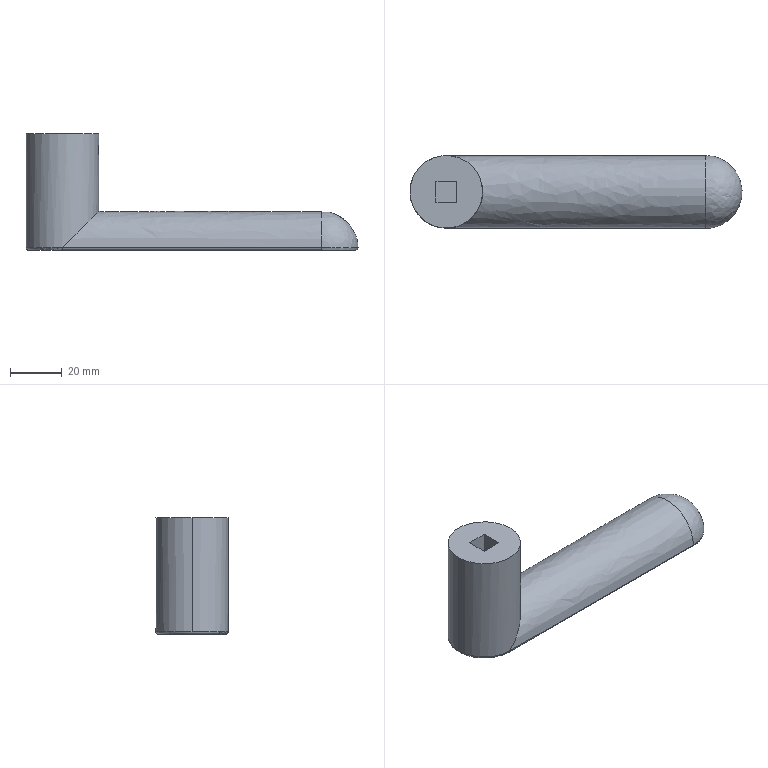Part | SolidWorks | features ICE 5, Cut 2, Blend 1, Extrusion 1, Fillet 1, HoleWzd 1, NetBlend 1 | 1 solid | 17 faces | box 128.025 x 28 x 45 mm | volume 59416 mm3 | plane 7 | cylinder 6 | spline 3 | torus 1 | commonest cylinder face diameters 2 x2 4.2 x2 28 x2
STEP:
#1=CARTESIAN_POINT('',(14.,0.,36.4));
#2=VERTEX_POINT('',#1);
#3=CARTESIAN_POINT('',(14.,0.,40.6));
#4=VERTEX_POINT('',#3);
#5=CARTESIAN_POINT('',(14.,0.,36.4));
#6=CARTESIAN_POINT('',(14.,-0.2742,36.4));
#7=CARTESIAN_POINT('',(13.991,-0.5509,36.455));
#8=CARTESIAN_POINT('',(13.97,-0.93,36.612));
#9=CARTESIAN_POINT('',(13.961,-1.052,36.677));
#10=CARTESIAN_POINT('',(13.942,-1.282,36.831));
#11=CARTESIAN_POINT('',(13.931,-1.387,36.917));
#12=CARTESIAN_POINT('',(13.911,-1.581,37.111));
#13=CARTESIAN_POINT('',(13.9,-1.669,37.219));
#14=CARTESIAN_POINT('',(13.881,-1.822,37.446));
#15=CARTESIAN_POINT('',(13.872,-1.886,37.567));
#16=CARTESIAN_POINT('',(13.858,-1.992,37.821));
#17=CARTESIAN_POINT('',(13.852,-2.033,37.954));
#18=CARTESIAN_POINT('',(13.844,-2.086,38.223));
#19=CARTESIAN_POINT('',(13.842,-2.1,38.36));
#20=CARTESIAN_POINT('',(13.842,-2.1,38.637));
#21=CARTESIAN_POINT('',(13.844,-2.087,38.774));
#22=CARTESIAN_POINT('',(13.852,-2.033,39.043));
#23=CARTESIAN_POINT('',(13.858,-1.993,39.176));
#24=CARTESIAN_POINT('',(13.872,-1.888,39.43));
#25=CARTESIAN_POINT('',(13.881,-1.823,39.551));
#26=CARTESIAN_POINT('',(13.9,-1.671,39.779));
#27=CARTESIAN_POINT('',(13.911,-1.583,39.887));
#28=CARTESIAN_POINT('',(13.942,-1.293,40.177));
#29=CARTESIAN_POINT('',(13.962,-1.059,40.334));
#30=CARTESIAN_POINT('',(13.991,-0.5539,40.544));
#31=CARTESIAN_POINT('',(14.,-0.2779,40.6));
#32=CARTESIAN_POINT('',(14.,0.,40.6));
#33=B_SPLINE_CURVE_WITH_KNOTS('',3,(#5,#6,#7,#8,#9,#10,#11,#12,#13,#14,#15,#16,#17,#18,#19,#20,#21,#22,#23,#24,#25,#26,#27,#28,#29,#30,#31,#32),.UNSPECIFIED.,.F.,.F.,(4,2,2,2,2,2,2,2,2,2,2,2,2,4),(0.006575,0.007396,0.007807,0.008218,0.008629,0.00904,0.009451,0.009861,0.01027,0.01068,0.01109,0.0115,0.01233,0.01315),.UNSPECIFIED.);
#34=EDGE_CURVE('',#2,#4,#33,.T.);
#35=ORIENTED_EDGE('',*,*,#34,.F.);
#36=CARTESIAN_POINT('',(4.,0.,36.4));
#37=VERTEX_POINT('',#36);
#38=CARTESIAN_POINT('',(4.,0.,36.4));
#39=DIRECTION('',(-1.,0.,0.));
#40=VECTOR('',#39,1000.);
#41=LINE('',#38,#40);
#42=EDGE_CURVE('',#2,#37,#41,.T.);
#43=ORIENTED_EDGE('',*,*,#42,.T.);
#44=CARTESIAN_POINT('',(4.,0.,40.6));
#45=VERTEX_POINT('',#44);
#46=CARTESIAN_POINT('',(4.,0.,38.5));
#47=DIRECTION('',(-1.,0.,0.));
#48=DIRECTION('',(0.,0.,1.));
#49=AXIS2_PLACEMENT_3D('',#46,#47,#48);
#50=CIRCLE('',#49,2.1);
#51=EDGE_CURVE('',#37,#45,#50,.T.);
#52=ORIENTED_EDGE('',*,*,#51,.T.);
#53=CARTESIAN_POINT('',(4.,0.,40.6));
#54=DIRECTION('',(-1.,0.,0.));
#55=VECTOR('',#54,1000.);
#56=LINE('',#53,#55);
#57=EDGE_CURVE('',#4,#45,#56,.T.);
#58=ORIENTED_EDGE('',*,*,#57,.F.);
#59=EDGE_LOOP('',(#35,#43,#52,#58));
#60=FACE_OUTER_BOUND('',#59,.T.);
#61=CARTESIAN_POINT('',(4.,0.,38.5));
#62=DIRECTION('',(-1.,0.,0.));
#63=DIRECTION('',(0.,0.,1.));
#64=AXIS2_PLACEMENT_3D('',#61,#62,#63);
#65=CYLINDRICAL_SURFACE('',#64,2.1);
#66=ADVANCED_FACE('',(#60),#65,.F.);
#67=CARTESIAN_POINT('',(14.,0.,45.));
#68=VERTEX_POINT('',#67);
#69=CARTESIAN_POINT('',(-14.,0.,45.));
#70=VERTEX_POINT('',#69);
#71=CARTESIAN_POINT('',(0.,0.,45.));
#72=DIRECTION('',(0.,0.,1.));
#73=DIRECTION('',(1.,0.,0.));
#74=AXIS2_PLACEMENT_3D('',#71,#72,#73);
#75=CIRCLE('',#74,14.);
#76=EDGE_CURVE('',#68,#70,#75,.T.);
#77=ORIENTED_EDGE('',*,*,#76,.F.);
#78=CARTESIAN_POINT('',(14.,0.,45.));
#79=DIRECTION('',(0.,0.,-1.));
#80=VECTOR('',#79,1000.);
#81=LINE('',#78,#80);
#82=EDGE_CURVE('',#68,#4,#81,.T.);
#83=ORIENTED_EDGE('',*,*,#82,.T.);
#84=CARTESIAN_POINT('',(14.,0.,40.6));
#85=CARTESIAN_POINT('',(14.,0.139,40.6));
#86=CARTESIAN_POINT('',(13.998,0.2756,40.586));
#87=CARTESIAN_POINT('',(13.99,0.5443,40.533));
#88=CARTESIAN_POINT('',(13.984,0.6777,40.492));
#89=CARTESIAN_POINT('',(13.97,0.932,40.387));
#90=CARTESIAN_POINT('',(13.961,1.053,40.322));
#91=CARTESIAN_POINT('',(13.942,1.281,40.17));
#92=CARTESIAN_POINT('',(13.931,1.389,40.081));
#93=CARTESIAN_POINT('',(13.9,1.679,39.791));
#94=CARTESIAN_POINT('',(13.88,1.835,39.557));
#95=CARTESIAN_POINT('',(13.85,2.045,39.052));
#96=CARTESIAN_POINT('',(13.842,2.1,38.775));
#97=CARTESIAN_POINT('',(13.842,2.1,38.364));
#98=CARTESIAN_POINT('',(13.844,2.086,38.224));
#99=CARTESIAN_POINT('',(13.852,2.033,37.955));
#100=CARTESIAN_POINT('',(13.858,1.993,37.824));
#101=CARTESIAN_POINT('',(13.872,1.887,37.569));
#102=CARTESIAN_POINT('',(13.881,1.822,37.447));
#103=CARTESIAN_POINT('',(13.9,1.67,37.219));
#104=CARTESIAN_POINT('',(13.911,1.583,37.113));
#105=CARTESIAN_POINT('',(13.931,1.387,36.917));
#106=CARTESIAN_POINT('',(13.942,1.281,36.831));
#107=CARTESIAN_POINT('',(13.961,1.054,36.679));
#108=CARTESIAN_POINT('',(13.97,0.9311,36.613));
#109=CARTESIAN_POINT('',(13.984,0.6769,36.507));
#110=CARTESIAN_POINT('',(13.99,0.546,36.468));
#111=CARTESIAN_POINT('',(13.998,0.2765,36.414));
#112=CARTESIAN_POINT('',(14.,0.1372,36.4));
#113=CARTESIAN_POINT('',(14.,0.,36.4));
#114=B_SPLINE_CURVE_WITH_KNOTS('',3,(#84,#85,#86,#87,#88,#89,#90,#91,#92,#93,#94,#95,#96,#97,#98,#99,#100,#101,#102,#103,#104,#105,#106,#107,#108,#109,#110,#111,#112,#113),.UNSPECIFIED.,.F.,.F.,(4,2,2,2,2,2,2,2,2,2,2,2,2,2,4),(0.,0.0004109,0.0008219,0.001233,0.001644,0.002466,0.003287,0.003698,0.004109,0.00452,0.004931,0.005342,0.005753,0.006164,0.006575),.UNSPECIFIED.);
#115=EDGE_CURVE('',#4,#2,#114,.T.);
#116=ORIENTED_EDGE('',*,*,#115,.T.);
#117=CARTESIAN_POINT('',(14.,0.,15.));
#118=VERTEX_POINT('',#117);
#119=CARTESIAN_POINT('',(14.,0.,45.));
#120=DIRECTION('',(0.,0.,-1.));
#121=VECTOR('',#120,1000.);
#122=LINE('',#119,#121);
#123=EDGE_CURVE('',#2,#118,#122,.T.);
#124=ORIENTED_EDGE('',*,*,#123,.T.);
#125=CARTESIAN_POINT('',(0.,14.,1.));
#126=VERTEX_POINT('',#125);
#127=CARTESIAN_POINT('',(14.,0.,15.));
#128=CARTESIAN_POINT('',(14.,0.5649,15.));
#129=CARTESIAN_POINT('',(13.966,1.123,14.966));
#130=CARTESIAN_POINT('',(13.833,2.228,14.832));
#131=CARTESIAN_POINT('',(13.733,2.777,14.732));
#132=CARTESIAN_POINT('',(13.475,3.836,14.475));
#133=CARTESIAN_POINT('',(13.318,4.347,14.319));
#134=CARTESIAN_POINT('',(13.045,5.088,14.046));
#135=CARTESIAN_POINT('',(12.948,5.331,13.949));
#136=CARTESIAN_POINT('',(12.741,5.808,13.741));
#137=CARTESIAN_POINT('',(12.631,6.044,13.631));
#138=CARTESIAN_POINT('',(12.057,7.189,13.056));
#139=CARTESIAN_POINT('',(11.524,8.007,12.523));
#140=CARTESIAN_POINT('',(10.637,9.115,11.637));
#141=CARTESIAN_POINT('',(10.325,9.466,11.325));
#142=CARTESIAN_POINT('',(9.683,10.122,10.684));
#143=CARTESIAN_POINT('',(9.354,10.426,10.354));
#144=CARTESIAN_POINT('',(8.342,11.278,9.341));
#145=CARTESIAN_POINT('',(7.636,11.764,8.635));
#146=CARTESIAN_POINT('',(6.537,12.387,7.537));
#147=CARTESIAN_POINT('',(6.162,12.578,7.163));
#148=CARTESIAN_POINT('',(5.411,12.918,6.413));
#149=CARTESIAN_POINT('',(5.034,13.07,6.035));
#150=CARTESIAN_POINT('',(3.895,13.471,4.895));
#151=CARTESIAN_POINT('',(3.129,13.669,4.126));
#152=CARTESIAN_POINT('',(1.578,13.933,2.573));
#153=CARTESIAN_POINT('',(0.7944,14.,1.79));
#154=CARTESIAN_POINT('',(0.,14.,1.));
#155=B_SPLINE_CURVE_WITH_KNOTS('',3,(#127,#128,#129,#130,#131,#132,#133,#134,#135,#136,#137,#138,#139,#140,#141,#142,#143,#144,#145,#146,#147,#148,#149,#150,#151,#152,#153,#154),.UNSPECIFIED.,.F.,.F.,(4,2,2,2,2,2,2,2,2,2,2,2,2,4),(0.02682,0.0285,0.03018,0.03186,0.0327,0.03354,0.0369,0.03858,0.04026,0.04362,0.0453,0.04698,0.05034,0.0537),.UNSPECIFIED.);
#156=EDGE_CURVE('',#118,#126,#155,.T.);
#157=ORIENTED_EDGE('',*,*,#156,.T.);
#158=CARTESIAN_POINT('',(-14.,0.,1.));
#159=VERTEX_POINT('',#158);
#160=CARTESIAN_POINT('',(0.,0.,1.));
#161=DIRECTION('',(0.,0.,1.));
#162=DIRECTION('',(1.,0.,0.));
#163=AXIS2_PLACEMENT_3D('',#160,#161,#162);
#164=CIRCLE('',#163,14.);
#165=EDGE_CURVE('',#126,#159,#164,.T.);
#166=ORIENTED_EDGE('',*,*,#165,.T.);
#167=CARTESIAN_POINT('',(-14.,0.,45.));
#168=DIRECTION('',(0.,0.,-1.));
#169=VECTOR('',#168,1000.);
#170=LINE('',#167,#169);
#171=EDGE_CURVE('',#70,#159,#170,.T.);
#172=ORIENTED_EDGE('',*,*,#171,.F.);
#173=EDGE_LOOP('',(#77,#83,#116,#124,#157,#166,#172));
#174=FACE_OUTER_BOUND('',#173,.T.);
#175=CARTESIAN_POINT('',(0.,0.,45.));
#176=DIRECTION('',(0.,0.,-1.));
#177=DIRECTION('',(-1.,0.,0.));
#178=AXIS2_PLACEMENT_3D('',#175,#176,#177);
#179=CYLINDRICAL_SURFACE('',#178,14.);
#180=ADVANCED_FACE('',(#174),#179,.T.);
#181=ORIENTED_EDGE('',*,*,#82,.F.);
#182=CARTESIAN_POINT('',(0.,0.,45.));
#183=DIRECTION('',(0.,0.,1.));
#184=DIRECTION('',(1.,0.,0.));
#185=AXIS2_PLACEMENT_3D('',#182,#183,#184);
#186=CIRCLE('',#185,14.);
#187=EDGE_CURVE('',#70,#68,#186,.T.);
#188=ORIENTED_EDGE('',*,*,#187,.F.);
#189=ORIENTED_EDGE('',*,*,#171,.T.);
#190=CARTESIAN_POINT('',(0.,-14.,1.));
#191=VERTEX_POINT('',#190);
#192=CARTESIAN_POINT('',(0.,0.,1.));
#193=DIRECTION('',(0.,0.,1.));
#194=DIRECTION('',(1.,0.,0.));
#195=AXIS2_PLACEMENT_3D('',#192,#193,#194);
#196=CIRCLE('',#195,14.);
#197=EDGE_CURVE('',#159,#191,#196,.T.);
#198=ORIENTED_EDGE('',*,*,#197,.T.);
#199=CARTESIAN_POINT('',(0.,-14.,1.));
#200=CARTESIAN_POINT('',(0.7932,-14.,1.789));
#201=CARTESIAN_POINT('',(1.584,-13.933,2.578));
#202=CARTESIAN_POINT('',(3.152,-13.664,4.149));
#203=CARTESIAN_POINT('',(3.929,-13.462,4.928));
#204=CARTESIAN_POINT('',(5.462,-12.916,6.464));
#205=CARTESIAN_POINT('',(6.209,-12.575,7.21));
#206=CARTESIAN_POINT('',(7.66,-11.748,8.659));
#207=CARTESIAN_POINT('',(8.363,-11.263,9.362));
#208=CARTESIAN_POINT('',(9.378,-10.404,10.378));
#209=CARTESIAN_POINT('',(9.71,-10.096,10.711));
#210=CARTESIAN_POINT('',(10.348,-9.441,11.348));
#211=CARTESIAN_POINT('',(10.654,-9.095,11.654));
#212=CARTESIAN_POINT('',(11.241,-8.359,12.24));
#213=CARTESIAN_POINT('',(11.52,-7.97,12.52));
#214=CARTESIAN_POINT('',(12.05,-7.144,13.049));
#215=CARTESIAN_POINT('',(12.301,-6.705,13.3));
#216=CARTESIAN_POINT('',(12.756,-5.792,13.756));
#217=CARTESIAN_POINT('',(12.961,-5.318,13.962));
#218=CARTESIAN_POINT('',(13.234,-4.576,14.234));
#219=CARTESIAN_POINT('',(13.318,-4.324,14.318));
#220=CARTESIAN_POINT('',(13.474,-3.809,14.474));
#221=CARTESIAN_POINT('',(13.546,-3.546,14.546));
#222=CARTESIAN_POINT('',(13.866,-2.22,14.865));
#223=CARTESIAN_POINT('',(14.,-1.128,15.));
#224=CARTESIAN_POINT('',(14.,0.,15.));
#225=B_SPLINE_CURVE_WITH_KNOTS('',3,(#199,#200,#201,#202,#203,#204,#205,#206,#207,#208,#209,#210,#211,#212,#213,#214,#215,#216,#217,#218,#219,#220,#221,#222,#223,#224),.UNSPECIFIED.,.F.,.F.,(4,2,2,2,2,2,2,2,2,2,2,2,4),(-0.00002366,0.003332,0.006687,0.01004,0.0134,0.01508,0.01675,0.01843,0.02011,0.02179,0.02263,0.02346,0.02682),.UNSPECIFIED.);
#226=EDGE_CURVE('',#191,#118,#225,.T.);
#227=ORIENTED_EDGE('',*,*,#226,.T.);
#228=ORIENTED_EDGE('',*,*,#123,.F.);
#229=ORIENTED_EDGE('',*,*,#34,.T.);
#230=EDGE_LOOP('',(#181,#188,#189,#198,#227,#228,#229));
#231=FACE_OUTER_BOUND('',#230,.T.);
#232=CARTESIAN_POINT('',(0.,0.,45.));
#233=DIRECTION('',(0.,0.,-1.));
#234=DIRECTION('',(-1.,0.,0.));
#235=AXIS2_PLACEMENT_3D('',#232,#233,#234);
#236=CYLINDRICAL_SURFACE('',#235,14.);
#237=ADVANCED_FACE('',(#231),#236,.T.);
#238=ORIENTED_EDGE('',*,*,#187,.T.);
#239=ORIENTED_EDGE('',*,*,#76,.T.);
#240=EDGE_LOOP('',(#238,#239));
#241=FACE_OUTER_BOUND('',#240,.T.);
#242=CARTESIAN_POINT('',(4.,-4.,45.));
#243=VERTEX_POINT('',#242);
#244=CARTESIAN_POINT('',(-4.,-4.,45.));
#245=VERTEX_POINT('',#244);
#246=CARTESIAN_POINT('',(-4.,-4.,45.));
#247=DIRECTION('',(-1.,0.,0.));
#248=VECTOR('',#247,1000.);
#249=LINE('',#246,#248);
#250=EDGE_CURVE('',#243,#245,#249,.T.);
#251=ORIENTED_EDGE('',*,*,#250,.T.);
#252=CARTESIAN_POINT('',(-4.,4.,45.));
#253=VERTEX_POINT('',#252);
#254=CARTESIAN_POINT('',(-4.,-4.,45.));
#255=DIRECTION('',(0.,1.,0.));
#256=VECTOR('',#255,1000.);
#257=LINE('',#254,#256);
#258=EDGE_CURVE('',#245,#253,#257,.T.);
#259=ORIENTED_EDGE('',*,*,#258,.T.);
#260=CARTESIAN_POINT('',(4.,4.,45.));
#261=VERTEX_POINT('',#260);
#262=CARTESIAN_POINT('',(-4.,4.,45.));
#263=DIRECTION('',(1.,0.,0.));
#264=VECTOR('',#263,1000.);
#265=LINE('',#262,#264);
#266=EDGE_CURVE('',#253,#261,#265,.T.);
#267=ORIENTED_EDGE('',*,*,#266,.T.);
#268=CARTESIAN_POINT('',(4.,-4.,45.));
#269=DIRECTION('',(0.,-1.,0.));
#270=VECTOR('',#269,1000.);
#271=LINE('',#268,#270);
#272=EDGE_CURVE('',#261,#243,#271,.T.);
#273=ORIENTED_EDGE('',*,*,#272,.T.);
#274=EDGE_LOOP('',(#251,#259,#267,#273));
#275=FACE_BOUND('',#274,.T.);
#276=CARTESIAN_POINT('',(0.,0.,45.));
#277=DIRECTION('',(0.,0.,1.));
#278=DIRECTION('',(1.,0.,0.));
#279=AXIS2_PLACEMENT_3D('',#276,#277,#278);
#280=PLANE('',#279);
#281=ADVANCED_FACE('',(#241,#275),#280,.T.);
#282=CARTESIAN_POINT('',(0.,13.,0.));
#283=VERTEX_POINT('',#282);
#284=CARTESIAN_POINT('',(99.976,13.,0.));
#285=VERTEX_POINT('',#284);
#286=CARTESIAN_POINT('',(100.,13.,0.));
#287=DIRECTION('',(1.,0.,0.));
#288=VECTOR('',#287,1000.);
#289=LINE('',#286,#288);
#290=EDGE_CURVE('',#283,#285,#289,.T.);
#291=ORIENTED_EDGE('',*,*,#290,.T.);
#292=CARTESIAN_POINT('',(99.977,-13.,0.));
#293=VERTEX_POINT('',#292);
#294=CARTESIAN_POINT('',(99.976,13.,0.));
#295=CARTESIAN_POINT('',(100.407,12.99,0.));
#296=CARTESIAN_POINT('',(100.838,12.982,0.));
#297=CARTESIAN_POINT('',(101.695,12.914,0.));
#298=CARTESIAN_POINT('',(102.123,12.858,0.));
#299=CARTESIAN_POINT('',(103.388,12.624,0.));
#300=CARTESIAN_POINT('',(104.203,12.383,0.));
#301=CARTESIAN_POINT('',(105.385,11.9,0.));
#302=CARTESIAN_POINT('',(105.773,11.718,0.));
#303=CARTESIAN_POINT('',(106.533,11.314,0.));
#304=CARTESIAN_POINT('',(106.9,11.094,0.));
#305=CARTESIAN_POINT('',(107.961,10.383,0.));
#306=CARTESIAN_POINT('',(108.618,9.843,0.));
#307=CARTESIAN_POINT('',(109.526,8.931,0.));
#308=CARTESIAN_POINT('',(109.815,8.61,0.));
#309=CARTESIAN_POINT('',(110.353,7.949,0.));
#310=CARTESIAN_POINT('',(110.605,7.606,0.));
#311=CARTESIAN_POINT('',(111.075,6.898,0.));
#312=CARTESIAN_POINT('',(111.293,6.533,0.));
#313=CARTESIAN_POINT('',(111.693,5.779,0.));
#314=CARTESIAN_POINT('',(111.877,5.388,0.));
#315=CARTESIAN_POINT('',(112.366,4.199,0.));
#316=CARTESIAN_POINT('',(112.609,3.386,0.));
#317=CARTESIAN_POINT('',(112.857,2.134,0.));
#318=CARTESIAN_POINT('',(112.92,1.711,0.));
#319=CARTESIAN_POINT('',(113.004,0.8554,0.));
#320=CARTESIAN_POINT('',(113.025,0.4269,0.));
#321=CARTESIAN_POINT('',(113.025,-0.8504,0.));
#322=CARTESIAN_POINT('',(112.94,-1.695,0.));
#323=CARTESIAN_POINT('',(112.691,-2.952,0.));
#324=CARTESIAN_POINT('',(112.587,-3.372,0.));
#325=CARTESIAN_POINT('',(112.34,-4.191,0.));
#326=CARTESIAN_POINT('',(112.198,-4.592,0.));
#327=CARTESIAN_POINT('',(111.714,-5.77,0.));
#328=CARTESIAN_POINT('',(111.316,-6.522,0.));
#329=CARTESIAN_POINT('',(110.365,-7.957,0.));
#330=CARTESIAN_POINT('',(109.827,-8.617,0.));
#331=CARTESIAN_POINT('',(108.93,-9.521,0.));
#332=CARTESIAN_POINT('',(108.616,-9.808,0.));
#333=CARTESIAN_POINT('',(107.957,-10.352,0.));
#334=CARTESIAN_POINT('',(107.61,-10.611,0.));
#335=CARTESIAN_POINT('',(106.546,-11.325,0.));
#336=CARTESIAN_POINT('',(105.798,-11.725,0.));
#337=CARTESIAN_POINT('',(104.223,-12.373,0.));
#338=CARTESIAN_POINT('',(103.392,-12.621,0.));
#339=CARTESIAN_POINT('',(102.125,-12.858,0.));
#340=CARTESIAN_POINT('',(101.697,-12.914,0.));
#341=CARTESIAN_POINT('',(100.839,-12.982,0.));
#342=CARTESIAN_POINT('',(100.408,-12.99,0.));
#343=CARTESIAN_POINT('',(99.977,-13.,0.));
#344=B_SPLINE_CURVE_WITH_KNOTS('',3,(#294,#295,#296,#297,#298,#299,#300,#301,#302,#303,#304,#305,#306,#307,#308,#309,#310,#311,#312,#313,#314,#315,#316,#317,#318,#319,#320,#321,#322,#323,#324,#325,#326,#327,#328,#329,#330,#331,#332,#333,#334,#335,#336,#337,#338,#339,#340,#341,#342,#343),.UNSPECIFIED.,.F.,.F.,(4,2,2,2,2,2,2,2,2,2,2,2,2,2,2,2,2,2,2,2,2,2,2,2,4),(0.,0.001292,0.002584,0.005168,0.00646,0.007752,0.01034,0.01163,0.01292,0.01421,0.0155,0.01809,0.01938,0.02067,0.02325,0.02455,0.02584,0.02842,0.03101,0.0323,0.03359,0.03617,0.03876,0.04005,0.04134),.UNSPECIFIED.);
#345=EDGE_CURVE('',#285,#293,#344,.T.);
#346=ORIENTED_EDGE('',*,*,#345,.T.);
#347=CARTESIAN_POINT('',(0.,-13.,0.));
#348=VERTEX_POINT('',#347);
#349=CARTESIAN_POINT('',(0.,-13.,0.));
#350=DIRECTION('',(-1.,0.,0.));
#351=VECTOR('',#350,1000.);
#352=LINE('',#349,#351);
#353=EDGE_CURVE('',#293,#348,#352,.T.);
#354=ORIENTED_EDGE('',*,*,#353,.T.);
#355=CARTESIAN_POINT('',(0.,0.,0.));
#356=DIRECTION('',(0.,0.,-1.));
#357=DIRECTION('',(1.,0.,0.));
#358=AXIS2_PLACEMENT_3D('',#355,#356,#357);
#359=CIRCLE('',#358,13.);
#360=EDGE_CURVE('',#348,#283,#359,.T.);
#361=ORIENTED_EDGE('',*,*,#360,.T.);
#362=EDGE_LOOP('',(#291,#346,#354,#361));
#363=FACE_OUTER_BOUND('',#362,.T.);
#364=CARTESIAN_POINT('',(0.,0.,0.));
#365=DIRECTION('',(0.,0.,1.));
#366=DIRECTION('',(1.,0.,0.));
#367=AXIS2_PLACEMENT_3D('',#364,#365,#366);
#368=PLANE('',#367);
#369=ADVANCED_FACE('',(#363),#368,.F.);
#370=CARTESIAN_POINT('',(100.,14.,1.));
#371=VERTEX_POINT('',#370);
#372=CARTESIAN_POINT('',(100.,-14.,1.));
#373=VERTEX_POINT('',#372);
#374=CARTESIAN_POINT('',(100.,0.,1.));
#375=DIRECTION('',(1.,0.,0.));
#376=DIRECTION('',(0.,0.,-1.));
#377=AXIS2_PLACEMENT_3D('',#374,#375,#376);
#378=CIRCLE('',#377,14.);
#379=EDGE_CURVE('',#371,#373,#378,.T.);
#380=ORIENTED_EDGE('',*,*,#379,.F.);
#381=CARTESIAN_POINT('',(100.,14.,1.));
#382=DIRECTION('',(-1.,0.,0.));
#383=VECTOR('',#382,1000.);
#384=LINE('',#381,#383);
#385=EDGE_CURVE('',#371,#126,#384,.T.);
#386=ORIENTED_EDGE('',*,*,#385,.T.);
#387=ORIENTED_EDGE('',*,*,#156,.F.);
#388=ORIENTED_EDGE('',*,*,#226,.F.);
#389=CARTESIAN_POINT('',(0.,-14.,1.));
#390=DIRECTION('',(1.,0.,0.));
#391=VECTOR('',#390,1000.);
#392=LINE('',#389,#391);
#393=EDGE_CURVE('',#191,#373,#392,.T.);
#394=ORIENTED_EDGE('',*,*,#393,.T.);
#395=EDGE_LOOP('',(#380,#386,#387,#388,#394));
#396=FACE_OUTER_BOUND('',#395,.T.);
#397=CARTESIAN_POINT('',(0.,14.,0.));
#398=CARTESIAN_POINT('',(100.,14.,0.));
#399=CARTESIAN_POINT('',(0.,14.,0.08333));
#400=CARTESIAN_POINT('',(100.,14.,0.08333));
#401=CARTESIAN_POINT('',(0.,14.,0.25));
#402=CARTESIAN_POINT('',(100.,14.,0.25));
#403=CARTESIAN_POINT('',(0.,14.,0.5));
#404=CARTESIAN_POINT('',(100.,14.,0.5));
#405=CARTESIAN_POINT('',(0.,14.,0.75));
#406=CARTESIAN_POINT('',(100.,14.,0.75));
#407=CARTESIAN_POINT('',(0.,14.,0.9167));
#408=CARTESIAN_POINT('',(100.,14.,0.9167));
#409=CARTESIAN_POINT('',(0.,14.,2.833));
#410=CARTESIAN_POINT('',(100.,14.,2.833));
#411=CARTESIAN_POINT('',(0.,13.272,6.497));
#412=CARTESIAN_POINT('',(100.,13.272,6.497));
#413=CARTESIAN_POINT('',(0.,10.157,11.158));
#414=CARTESIAN_POINT('',(100.,10.157,11.158));
#415=CARTESIAN_POINT('',(0.,5.497,14.271));
#416=CARTESIAN_POINT('',(100.,5.497,14.271));
#417=CARTESIAN_POINT('',(0.,0.,15.365));
#418=CARTESIAN_POINT('',(100.,0.,15.365));
#419=CARTESIAN_POINT('',(0.,-5.497,14.271));
#420=CARTESIAN_POINT('',(100.,-5.497,14.271));
#421=CARTESIAN_POINT('',(0.,-10.157,11.158));
#422=CARTESIAN_POINT('',(100.,-10.157,11.158));
#423=CARTESIAN_POINT('',(0.,-13.272,6.497));
#424=CARTESIAN_POINT('',(100.,-13.272,6.497));
#425=CARTESIAN_POINT('',(0.,-14.,2.833));
#426=CARTESIAN_POINT('',(100.,-14.,2.833));
#427=CARTESIAN_POINT('',(0.,-14.,0.9167));
#428=CARTESIAN_POINT('',(100.,-14.,0.9167));
#429=CARTESIAN_POINT('',(0.,-14.,0.75));
#430=CARTESIAN_POINT('',(100.,-14.,0.75));
#431=CARTESIAN_POINT('',(0.,-14.,0.5));
#432=CARTESIAN_POINT('',(100.,-14.,0.5));
#433=CARTESIAN_POINT('',(0.,-14.,0.25));
#434=CARTESIAN_POINT('',(100.,-14.,0.25));
#435=CARTESIAN_POINT('',(0.,-14.,0.08333));
#436=CARTESIAN_POINT('',(100.,-14.,0.08333));
#437=CARTESIAN_POINT('',(0.,-14.,0.));
#438=CARTESIAN_POINT('',(100.,-14.,0.));
#439=B_SPLINE_SURFACE_WITH_KNOTS('',3,1,((#397,#398),(#399,#400),(#401,#402),(#403,#404),(#405,#406),(#407,#408),(#409,#410),(#411,#412),(#413,#414),(#415,#416),(#417,#418),(#419,#420),(#421,#422),(#423,#424),(#425,#426),(#427,#428),(#429,#430),(#431,#432),(#433,#434),(#435,#436),(#437,#438)),.UNSPECIFIED.,.F.,.F.,.F.,(4,1,1,1,2,1,1,1,1,1,1,1,2,1,1,1,4),(2,2),(0.,0.005437,0.01087,0.01631,0.02175,0.1413,0.2609,0.3804,0.5,0.6196,0.7391,0.8587,0.9783,0.9837,0.9891,0.9946,1.),(0.,1.),.UNSPECIFIED.);
#440=ADVANCED_FACE('',(#396),#439,.T.);
#441=ORIENTED_EDGE('',*,*,#379,.T.);
#442=CARTESIAN_POINT('',(100.313,-13.993,1.006));
#443=VERTEX_POINT('',#442);
#444=CARTESIAN_POINT('',(100.,-14.,1.));
#445=CARTESIAN_POINT('',(100.,-14.,1.));
#446=CARTESIAN_POINT('',(100.,-14.,1.));
#447=CARTESIAN_POINT('',(100.,-14.,1.));
#448=CARTESIAN_POINT('',(100.025,-13.999,1.001));
#449=CARTESIAN_POINT('',(100.049,-13.999,1.001));
#450=CARTESIAN_POINT('',(100.073,-13.998,1.002));
#451=CARTESIAN_POINT('',(100.153,-13.997,1.003));
#452=CARTESIAN_POINT('',(100.233,-13.995,1.005));
#453=CARTESIAN_POINT('',(100.313,-13.993,1.006));
#454=CARTESIAN_POINT('',(100.313,-13.993,1.006));
#455=CARTESIAN_POINT('',(100.313,-13.993,1.006));
#456=CARTESIAN_POINT('',(100.313,-13.993,1.006));
#457=B_SPLINE_CURVE_WITH_KNOTS('',3,(#444,#445,#446,#447,#448,#449,#450,#451,#452,#453,#454,#455,#456),.UNSPECIFIED.,.F.,.F.,(4,3,3,3,4),(-0.00000006,0.,0.00007337,0.0003131,0.0003132),.UNSPECIFIED.);
#458=EDGE_CURVE('',#373,#443,#457,.T.);
#459=ORIENTED_EDGE('',*,*,#458,.T.);
#460=CARTESIAN_POINT('',(100.339,13.992,1.007));
#461=VERTEX_POINT('',#460);
#462=CARTESIAN_POINT('',(100.313,-13.993,1.006));
#463=CARTESIAN_POINT('',(100.541,-13.988,1.012));
#464=CARTESIAN_POINT('',(100.769,-13.981,1.018));
#465=CARTESIAN_POINT('',(101.225,-13.956,1.022));
#466=CARTESIAN_POINT('',(101.452,-13.938,1.021));
#467=CARTESIAN_POINT('',(102.133,-13.867,1.017));
#468=CARTESIAN_POINT('',(102.584,-13.796,1.011));
#469=CARTESIAN_POINT('',(103.475,-13.609,1.001));
#470=CARTESIAN_POINT('',(103.916,-13.492,0.9974));
#471=CARTESIAN_POINT('',(104.784,-13.215,0.9912));
#472=CARTESIAN_POINT('',(105.208,-13.056,0.989));
#473=CARTESIAN_POINT('',(106.448,-12.519,0.9843));
#474=CARTESIAN_POINT('',(107.234,-12.081,0.9837));
#475=CARTESIAN_POINT('',(108.353,-11.307,0.9851));
#476=CARTESIAN_POINT('',(108.716,-11.028,0.986));
#477=CARTESIAN_POINT('',(109.406,-10.443,0.9881));
#478=CARTESIAN_POINT('',(109.735,-10.135,0.9894));
#479=CARTESIAN_POINT('',(110.362,-9.489,0.9922));
#480=CARTESIAN_POINT('',(110.659,-9.152,0.9938));
#481=CARTESIAN_POINT('',(111.222,-8.447,0.9969));
#482=CARTESIAN_POINT('',(111.488,-8.078,0.9986));
#483=CARTESIAN_POINT('',(112.234,-6.933,1.003));
#484=CARTESIAN_POINT('',(112.65,-6.133,1.006));
#485=CARTESIAN_POINT('',(113.157,-4.882,1.009));
#486=CARTESIAN_POINT('',(113.306,-4.456,1.01));
#487=CARTESIAN_POINT('',(113.565,-3.587,1.012));
#488=CARTESIAN_POINT('',(113.674,-3.142,1.012));
#489=CARTESIAN_POINT('',(113.848,-2.254,1.013));
#490=CARTESIAN_POINT('',(113.913,-1.808,1.013));
#491=CARTESIAN_POINT('',(114.001,-0.9128,1.013));
#492=CARTESIAN_POINT('',(114.024,-0.4635,1.011));
#493=CARTESIAN_POINT('',(114.025,0.4387,1.011));
#494=CARTESIAN_POINT('',(114.004,0.8925,1.011));
#495=CARTESIAN_POINT('',(113.917,1.8,1.01));
#496=CARTESIAN_POINT('',(113.852,2.248,1.01));
#497=CARTESIAN_POINT('',(113.595,3.576,1.008));
#498=CARTESIAN_POINT('',(113.341,4.44,1.006));
#499=CARTESIAN_POINT('',(112.832,5.702,1.002));
#500=CARTESIAN_POINT('',(112.641,6.118,1.));
#501=CARTESIAN_POINT('',(112.223,6.921,0.997));
#502=CARTESIAN_POINT('',(111.768,7.7,0.9937));
#503=CARTESIAN_POINT('',(111.242,8.431,0.9905));
#504=CARTESIAN_POINT('',(110.68,9.138,0.9874));
#505=CARTESIAN_POINT('',(110.379,9.481,0.986));
#506=CARTESIAN_POINT('',(109.428,10.462,0.982));
#507=CARTESIAN_POINT('',(108.74,11.045,0.9802));
#508=CARTESIAN_POINT('',(107.629,11.815,0.9797));
#509=CARTESIAN_POINT('',(107.245,12.055,0.98));
#510=CARTESIAN_POINT('',(106.45,12.497,0.9815));
#511=CARTESIAN_POINT('',(106.041,12.699,0.9828));
#512=CARTESIAN_POINT('',(104.796,13.237,0.9888));
#513=CARTESIAN_POINT('',(103.939,13.511,0.9958));
#514=CARTESIAN_POINT('',(102.61,13.792,1.011));
#515=CARTESIAN_POINT('',(102.158,13.864,1.017));
#516=CARTESIAN_POINT('',(101.478,13.936,1.022));
#517=CARTESIAN_POINT('',(101.251,13.954,1.022));
#518=CARTESIAN_POINT('',(100.796,13.979,1.019));
#519=CARTESIAN_POINT('',(100.568,13.987,1.013));
#520=CARTESIAN_POINT('',(100.339,13.992,1.007));
#521=B_SPLINE_CURVE_WITH_KNOTS('',3,(#462,#463,#464,#465,#466,#467,#468,#469,#470,#471,#472,#473,#474,#475,#476,#477,#478,#479,#480,#481,#482,#483,#484,#485,#486,#487,#488,#489,#490,#491,#492,#493,#494,#495,#496,#497,#498,#499,#500,#501,#502,#503,#504,#505,#506,#507,#508,#509,#510,#511,#512,#513,#514,#515,#516,#517,#518,#519,#520),.UNSPECIFIED.,.F.,.F.,(4,2,2,2,2,2,2,2,2,2,2,2,2,2,2,2,2,2,2,2,1,2,2,2,2,2,2,2,2,4),(-0.00000006,0.0006846,0.001369,0.002739,0.004108,0.005477,0.008216,0.009585,0.01095,0.01232,0.01369,0.01643,0.0178,0.01917,0.02054,0.02191,0.02328,0.02465,0.02739,0.02876,0.03013,0.03149,0.03286,0.0356,0.03697,0.03834,0.04108,0.04245,0.04313,0.04382),.UNSPECIFIED.);
#522=EDGE_CURVE('',#443,#461,#521,.T.);
#523=ORIENTED_EDGE('',*,*,#522,.T.);
#524=CARTESIAN_POINT('',(100.339,13.992,1.007));
#525=CARTESIAN_POINT('',(100.339,13.992,1.007));
#526=CARTESIAN_POINT('',(100.339,13.992,1.007));
#527=CARTESIAN_POINT('',(100.339,13.992,1.007));
#528=CARTESIAN_POINT('',(100.268,13.994,1.006));
#529=CARTESIAN_POINT('',(100.197,13.995,1.004));
#530=CARTESIAN_POINT('',(100.126,13.997,1.003));
#531=CARTESIAN_POINT('',(100.092,13.998,1.002));
#532=CARTESIAN_POINT('',(100.059,13.999,1.001));
#533=CARTESIAN_POINT('',(100.025,13.999,1.001));
#534=CARTESIAN_POINT('',(100.017,14.,1.));
#535=CARTESIAN_POINT('',(100.008,14.,1.));
#536=CARTESIAN_POINT('',(100.,14.,1.));
#537=CARTESIAN_POINT('',(100.,14.,1.));
#538=CARTESIAN_POINT('',(100.,14.,1.));
#539=CARTESIAN_POINT('',(100.,14.,1.));
#540=B_SPLINE_CURVE_WITH_KNOTS('',3,(#524,#525,#526,#527,#528,#529,#530,#531,#532,#533,#534,#535,#536,#537,#538,#539),.UNSPECIFIED.,.F.,.F.,(4,3,3,3,3,4),(-0.00000006,0.,0.0002138,0.0003145,0.0003395,0.0003396),.UNSPECIFIED.);
#541=EDGE_CURVE('',#461,#371,#540,.T.);
#542=ORIENTED_EDGE('',*,*,#541,.T.);
#543=EDGE_LOOP('',(#441,#459,#523,#542));
#544=FACE_OUTER_BOUND('',#543,.T.);
#545=CARTESIAN_POINT('',(100.,14.,0.));
#546=CARTESIAN_POINT('',(100.,14.,0.));
#547=CARTESIAN_POINT('',(100.,14.,0.));
#548=CARTESIAN_POINT('',(100.,14.,0.));
#549=CARTESIAN_POINT('',(100.,14.,0.));
#550=CARTESIAN_POINT('',(100.,14.,0.));
#551=CARTESIAN_POINT('',(100.,14.,0.));
#552=CARTESIAN_POINT('',(100.087,14.,0.));
#553=CARTESIAN_POINT('',(100.09,14.,0.0118));
#554=CARTESIAN_POINT('',(100.089,14.,0.03614));
#555=CARTESIAN_POINT('',(100.071,14.,0.06711));
#556=CARTESIAN_POINT('',(100.039,14.,0.08576));
#557=CARTESIAN_POINT('',(100.013,14.,0.08677));
#558=CARTESIAN_POINT('',(100.,14.,0.08408));
#559=CARTESIAN_POINT('',(100.265,13.998,0.));
#560=CARTESIAN_POINT('',(100.273,13.999,0.0351));
#561=CARTESIAN_POINT('',(100.269,13.999,0.1075));
#562=CARTESIAN_POINT('',(100.213,13.999,0.1997));
#563=CARTESIAN_POINT('',(100.117,14.,0.255));
#564=CARTESIAN_POINT('',(100.039,14.,0.2577));
#565=CARTESIAN_POINT('',(100.,14.,0.2495));
#566=CARTESIAN_POINT('',(100.534,13.991,0.));
#567=CARTESIAN_POINT('',(100.549,13.992,0.06965));
#568=CARTESIAN_POINT('',(100.541,13.993,0.2134));
#569=CARTESIAN_POINT('',(100.427,13.995,0.3963));
#570=CARTESIAN_POINT('',(100.234,13.998,0.506));
#571=CARTESIAN_POINT('',(100.078,13.999,0.5113));
#572=CARTESIAN_POINT('',(100.,14.,0.4949));
#573=CARTESIAN_POINT('',(100.801,13.978,0.));
#574=CARTESIAN_POINT('',(100.822,13.98,0.1043));
#575=CARTESIAN_POINT('',(100.81,13.984,0.3194));
#576=CARTESIAN_POINT('',(100.638,13.989,0.5932));
#577=CARTESIAN_POINT('',(100.349,13.994,0.7578));
#578=CARTESIAN_POINT('',(100.116,13.998,0.7665));
#579=CARTESIAN_POINT('',(100.,14.,0.7425));
#580=CARTESIAN_POINT('',(100.972,13.966,0.));
#581=CARTESIAN_POINT('',(100.999,13.97,0.1277));
#582=CARTESIAN_POINT('',(100.984,13.975,0.3909));
#583=CARTESIAN_POINT('',(100.776,13.983,0.726));
#584=CARTESIAN_POINT('',(100.425,13.991,0.9284));
#585=CARTESIAN_POINT('',(100.141,13.997,0.9404));
#586=CARTESIAN_POINT('',(100.,14.,0.912));
#587=CARTESIAN_POINT('',(102.8,13.828,0.));
#588=CARTESIAN_POINT('',(102.881,13.844,0.3883));
#589=CARTESIAN_POINT('',(102.847,13.873,1.186));
#590=CARTESIAN_POINT('',(102.247,13.914,2.205));
#591=CARTESIAN_POINT('',(101.232,13.955,2.835));
#592=CARTESIAN_POINT('',(100.409,13.984,2.897));
#593=CARTESIAN_POINT('',(100.,14.,2.828));
#594=CARTESIAN_POINT('',(106.218,12.907,0.));
#595=CARTESIAN_POINT('',(106.357,12.941,0.8672));
#596=CARTESIAN_POINT('',(106.227,13.003,2.639));
#597=CARTESIAN_POINT('',(104.888,13.09,4.913));
#598=CARTESIAN_POINT('',(102.675,13.177,6.371));
#599=CARTESIAN_POINT('',(100.889,13.24,6.597));
#600=CARTESIAN_POINT('',(100.,13.273,6.505));
#601=CARTESIAN_POINT('',(110.478,9.769,0.));
#602=CARTESIAN_POINT('',(110.625,9.802,1.449));
#603=CARTESIAN_POINT('',(110.29,9.864,4.392));
#604=CARTESIAN_POINT('',(108.017,9.95,8.188));
#605=CARTESIAN_POINT('',(104.378,10.036,10.71));
#606=CARTESIAN_POINT('',(101.459,10.097,11.241));
#607=CARTESIAN_POINT('',(100.,10.13,11.191));
#608=CARTESIAN_POINT('',(113.321,5.285,0.));
#609=CARTESIAN_POINT('',(113.446,5.299,1.824));
#610=CARTESIAN_POINT('',(112.94,5.326,5.52));
#611=CARTESIAN_POINT('',(110.037,5.364,10.298));
#612=CARTESIAN_POINT('',(105.475,5.401,13.527));
#613=CARTESIAN_POINT('',(101.827,5.428,14.291));
#614=CARTESIAN_POINT('',(100.,5.442,14.293));
#615=CARTESIAN_POINT('',(114.008,1.73,0.));
#616=CARTESIAN_POINT('',(114.124,1.733,1.911));
#617=CARTESIAN_POINT('',(113.571,1.738,5.779));
#618=CARTESIAN_POINT('',(110.516,1.745,10.782));
#619=CARTESIAN_POINT('',(105.735,1.752,14.174));
#620=CARTESIAN_POINT('',(101.914,1.757,14.993));
#621=CARTESIAN_POINT('',(100.,1.759,15.009));
#622=CARTESIAN_POINT('',(114.,-0.1294,0.));
#623=CARTESIAN_POINT('',(114.115,-0.1296,1.909));
#624=CARTESIAN_POINT('',(113.563,-0.1299,5.775));
#625=CARTESIAN_POINT('',(110.51,-0.1305,10.776));
#626=CARTESIAN_POINT('',(105.731,-0.131,14.166));
#627=CARTESIAN_POINT('',(101.913,-0.1314,14.984));
#628=CARTESIAN_POINT('',(100.,-0.1316,15.));
#629=CARTESIAN_POINT('',(113.995,-0.4287,0.));
#630=CARTESIAN_POINT('',(114.111,-0.3974,1.909));
#631=CARTESIAN_POINT('',(113.559,-0.3392,5.775));
#632=CARTESIAN_POINT('',(110.507,-0.2583,10.776));
#633=CARTESIAN_POINT('',(105.73,-0.1774,14.166));
#634=CARTESIAN_POINT('',(101.912,-0.1192,14.984));
#635=CARTESIAN_POINT('',(100.,-0.088,15.));
#636=CARTESIAN_POINT('',(113.983,-0.6973,0.));
#637=CARTESIAN_POINT('',(114.1,-0.6454,1.909));
#638=CARTESIAN_POINT('',(113.55,-0.5485,5.775));
#639=CARTESIAN_POINT('',(110.501,-0.4139,10.775));
#640=CARTESIAN_POINT('',(105.727,-0.2792,14.165));
#641=CARTESIAN_POINT('',(101.911,-0.1824,14.983));
#642=CARTESIAN_POINT('',(100.,-0.1304,14.999));
#643=CARTESIAN_POINT('',(113.976,-0.8133,0.));
#644=CARTESIAN_POINT('',(114.094,-0.7507,1.909));
#645=CARTESIAN_POINT('',(113.544,-0.6341,5.775));
#646=CARTESIAN_POINT('',(110.497,-0.472,10.774));
#647=CARTESIAN_POINT('',(105.725,-0.3099,14.164));
#648=CARTESIAN_POINT('',(101.911,-0.1934,14.983));
#649=CARTESIAN_POINT('',(100.,-0.1308,14.999));
#650=CARTESIAN_POINT('',(113.87,-2.557,0.));
#651=CARTESIAN_POINT('',(113.992,-2.503,1.905));
#652=CARTESIAN_POINT('',(113.453,-2.402,5.762));
#653=CARTESIAN_POINT('',(110.43,-2.26,10.751));
#654=CARTESIAN_POINT('',(105.689,-2.119,14.136));
#655=CARTESIAN_POINT('',(101.898,-2.018,14.957));
#656=CARTESIAN_POINT('',(100.,-1.963,14.977));
#657=CARTESIAN_POINT('',(113.037,-5.889,0.));
#658=CARTESIAN_POINT('',(113.175,-5.859,1.814));
#659=CARTESIAN_POINT('',(112.699,-5.803,5.488));
#660=CARTESIAN_POINT('',(109.862,-5.726,10.239));
#661=CARTESIAN_POINT('',(105.381,-5.649,13.456));
#662=CARTESIAN_POINT('',(101.795,-5.593,14.226));
#663=CARTESIAN_POINT('',(100.,-5.563,14.237));
#664=CARTESIAN_POINT('',(110.143,-10.081,0.));
#665=CARTESIAN_POINT('',(110.303,-10.091,1.436));
#666=CARTESIAN_POINT('',(110.003,-10.109,4.352));
#667=CARTESIAN_POINT('',(107.806,-10.135,8.114));
#668=CARTESIAN_POINT('',(104.265,-10.16,10.622));
#669=CARTESIAN_POINT('',(101.42,-10.179,11.163));
#670=CARTESIAN_POINT('',(100.,-10.189,11.124));
#671=CARTESIAN_POINT('',(105.984,-12.989,0.));
#672=CARTESIAN_POINT('',(106.131,-13.016,0.8579));
#673=CARTESIAN_POINT('',(106.022,-13.067,2.609));
#674=CARTESIAN_POINT('',(104.736,-13.137,4.858));
#675=CARTESIAN_POINT('',(102.593,-13.207,6.307));
#676=CARTESIAN_POINT('',(100.861,-13.258,6.545));
#677=CARTESIAN_POINT('',(100.,-13.285,6.462));
#678=CARTESIAN_POINT('',(102.697,-13.84,0.));
#679=CARTESIAN_POINT('',(102.78,-13.855,0.3843));
#680=CARTESIAN_POINT('',(102.755,-13.882,1.173));
#681=CARTESIAN_POINT('',(102.178,-13.92,2.182));
#682=CARTESIAN_POINT('',(101.194,-13.958,2.809));
#683=CARTESIAN_POINT('',(100.396,-13.985,2.877));
#684=CARTESIAN_POINT('',(100.,-14.,2.814));
#685=CARTESIAN_POINT('',(100.94,-13.969,0.));
#686=CARTESIAN_POINT('',(100.967,-13.972,0.1269));
#687=CARTESIAN_POINT('',(100.956,-13.977,0.3883));
#688=CARTESIAN_POINT('',(100.754,-13.984,0.7215));
#689=CARTESIAN_POINT('',(100.413,-13.992,0.9241));
#690=CARTESIAN_POINT('',(100.137,-13.997,0.9386));
#691=CARTESIAN_POINT('',(100.,-14.,0.9122));
#692=CARTESIAN_POINT('',(100.775,-13.979,0.));
#693=CARTESIAN_POINT('',(100.797,-13.981,0.1036));
#694=CARTESIAN_POINT('',(100.787,-13.985,0.3171));
#695=CARTESIAN_POINT('',(100.621,-13.99,0.5891));
#696=CARTESIAN_POINT('',(100.34,-13.995,0.7538));
#697=CARTESIAN_POINT('',(100.113,-13.998,0.7645));
#698=CARTESIAN_POINT('',(100.,-14.,0.742));
#699=CARTESIAN_POINT('',(100.519,-13.991,0.));
#700=CARTESIAN_POINT('',(100.534,-13.992,0.06903));
#701=CARTESIAN_POINT('',(100.527,-13.993,0.2114));
#702=CARTESIAN_POINT('',(100.416,-13.996,0.3926));
#703=CARTESIAN_POINT('',(100.228,-13.998,0.502));
#704=CARTESIAN_POINT('',(100.076,-13.999,0.5083));
#705=CARTESIAN_POINT('',(100.,-14.,0.4928));
#706=CARTESIAN_POINT('',(100.259,-13.998,0.));
#707=CARTESIAN_POINT('',(100.267,-13.999,0.03462));
#708=CARTESIAN_POINT('',(100.264,-13.999,0.1061));
#709=CARTESIAN_POINT('',(100.208,-13.999,0.197));
#710=CARTESIAN_POINT('',(100.114,-14.,0.2517));
#711=CARTESIAN_POINT('',(100.038,-14.,0.2546));
#712=CARTESIAN_POINT('',(100.,-14.,0.2467));
#713=CARTESIAN_POINT('',(100.086,-14.,0.));
#714=CARTESIAN_POINT('',(100.089,-14.,0.01159));
#715=CARTESIAN_POINT('',(100.088,-14.,0.0355));
#716=CARTESIAN_POINT('',(100.069,-14.,0.06592));
#717=CARTESIAN_POINT('',(100.038,-14.,0.08424));
#718=CARTESIAN_POINT('',(100.013,-14.,0.08524));
#719=CARTESIAN_POINT('',(100.,-14.,0.08259));
#720=CARTESIAN_POINT('',(100.,-14.,0.));
#721=CARTESIAN_POINT('',(100.,-14.,0.));
#722=CARTESIAN_POINT('',(100.,-14.,0.));
#723=CARTESIAN_POINT('',(100.,-14.,0.));
#724=CARTESIAN_POINT('',(100.,-14.,0.));
#725=CARTESIAN_POINT('',(100.,-14.,0.));
#726=CARTESIAN_POINT('',(100.,-14.,0.));
#727=B_SPLINE_SURFACE_WITH_KNOTS('',3,3,((#545,#546,#547,#548,#549,#550,#551),(#552,#553,#554,#555,#556,#557,#558),(#559,#560,#561,#562,#563,#564,#565),(#566,#567,#568,#569,#570,#571,#572),(#573,#574,#575,#576,#577,#578,#579),(#580,#581,#582,#583,#584,#585,#586),(#587,#588,#589,#590,#591,#592,#593),(#594,#595,#596,#597,#598,#599,#600),(#601,#602,#603,#604,#605,#606,#607),(#608,#609,#610,#611,#612,#613,#614),(#615,#616,#617,#618,#619,#620,#621),(#622,#623,#624,#625,#626,#627,#628),(#629,#630,#631,#632,#633,#634,#635),(#636,#637,#638,#639,#640,#641,#642),(#643,#644,#645,#646,#647,#648,#649),(#650,#651,#652,#653,#654,#655,#656),(#657,#658,#659,#660,#661,#662,#663),(#664,#665,#666,#667,#668,#669,#670),(#671,#672,#673,#674,#675,#676,#677),(#678,#679,#680,#681,#682,#683,#684),(#685,#686,#687,#688,#689,#690,#691),(#692,#693,#694,#695,#696,#697,#698),(#699,#700,#701,#702,#703,#704,#705),(#706,#707,#708,#709,#710,#711,#712),(#713,#714,#715,#716,#717,#718,#719),(#720,#721,#722,#723,#724,#725,#726)),.UNSPECIFIED.,.F.,.F.,.F.,(4,1,1,1,2,1,1,1,1,1,1,1,2,1,1,1,2,1,1,1,4),(4,1,1,1,4),(0.6919,0.6954,0.6989,0.7025,0.706,0.7795,0.853,0.9265,1.,1.002,1.004,1.005,1.007,1.079,1.151,1.222,1.294,1.298,1.301,1.305,1.308),(0.,0.25,0.5,0.75,1.),.UNSPECIFIED.);
#728=ADVANCED_FACE('',(#544),#727,.F.);
#729=CARTESIAN_POINT('',(4.,-4.,30.6));
#730=VERTEX_POINT('',#729);
#731=CARTESIAN_POINT('',(4.,4.,30.6));
#732=VERTEX_POINT('',#731);
#733=CARTESIAN_POINT('',(4.,-4.,30.6));
#734=DIRECTION('',(0.,1.,0.));
#735=VECTOR('',#734,1000.);
#736=LINE('',#733,#735);
#737=EDGE_CURVE('',#730,#732,#736,.T.);
#738=ORIENTED_EDGE('',*,*,#737,.T.);
#739=CARTESIAN_POINT('',(-4.,4.,30.6));
#740=VERTEX_POINT('',#739);
#741=CARTESIAN_POINT('',(-4.,4.,30.6));
#742=DIRECTION('',(-1.,0.,0.));
#743=VECTOR('',#742,1000.);
#744=LINE('',#741,#743);
#745=EDGE_CURVE('',#732,#740,#744,.T.);
#746=ORIENTED_EDGE('',*,*,#745,.T.);
#747=CARTESIAN_POINT('',(-4.,-4.,30.6));
#748=VERTEX_POINT('',#747);
#749=CARTESIAN_POINT('',(-4.,-4.,30.6));
#750=DIRECTION('',(0.,-1.,0.));
#751=VECTOR('',#750,1000.);
#752=LINE('',#749,#751);
#753=EDGE_CURVE('',#740,#748,#752,.T.);
#754=ORIENTED_EDGE('',*,*,#753,.T.);
#755=CARTESIAN_POINT('',(-4.,-4.,30.6));
#756=DIRECTION('',(1.,0.,0.));
#757=VECTOR('',#756,1000.);
#758=LINE('',#755,#757);
#759=EDGE_CURVE('',#748,#730,#758,.T.);
#760=ORIENTED_EDGE('',*,*,#759,.T.);
#761=EDGE_LOOP('',(#738,#746,#754,#760));
#762=FACE_OUTER_BOUND('',#761,.T.);
#763=CARTESIAN_POINT('',(0.,0.,30.6));
#764=DIRECTION('',(0.,0.,-1.));
#765=DIRECTION('',(-1.,0.,0.));
#766=AXIS2_PLACEMENT_3D('',#763,#764,#765);
#767=PLANE('',#766);
#768=ADVANCED_FACE('',(#762),#767,.F.);
#769=ORIENTED_EDGE('',*,*,#266,.F.);
#770=CARTESIAN_POINT('',(-4.,4.,30.6));
#771=DIRECTION('',(0.,0.,1.));
#772=VECTOR('',#771,1000.);
#773=LINE('',#770,#772);
#774=EDGE_CURVE('',#740,#253,#773,.T.);
#775=ORIENTED_EDGE('',*,*,#774,.F.);
#776=ORIENTED_EDGE('',*,*,#745,.F.);
#777=CARTESIAN_POINT('',(4.,4.,30.6));
#778=DIRECTION('',(0.,0.,1.));
#779=VECTOR('',#778,1000.);
#780=LINE('',#777,#779);
#781=EDGE_CURVE('',#732,#261,#780,.T.);
#782=ORIENTED_EDGE('',*,*,#781,.T.);
#783=EDGE_LOOP('',(#769,#775,#776,#782));
#784=FACE_OUTER_BOUND('',#783,.T.);
#785=CARTESIAN_POINT('',(-4.,4.,30.6));
#786=DIRECTION('',(0.,1.,0.));
#787=DIRECTION('',(0.,0.,1.));
#788=AXIS2_PLACEMENT_3D('',#785,#786,#787);
#789=PLANE('',#788);
#790=ADVANCED_FACE('',(#784),#789,.F.);
#791=ORIENTED_EDGE('',*,*,#250,.F.);
#792=CARTESIAN_POINT('',(4.,-4.,30.6));
#793=DIRECTION('',(0.,0.,1.));
#794=VECTOR('',#793,1000.);
#795=LINE('',#792,#794);
#796=EDGE_CURVE('',#730,#243,#795,.T.);
#797=ORIENTED_EDGE('',*,*,#796,.F.);
#798=ORIENTED_EDGE('',*,*,#759,.F.);
#799=CARTESIAN_POINT('',(-4.,-4.,30.6));
#800=DIRECTION('',(0.,0.,1.));
#801=VECTOR('',#800,1000.);
#802=LINE('',#799,#801);
#803=EDGE_CURVE('',#748,#245,#802,.T.);
#804=ORIENTED_EDGE('',*,*,#803,.T.);
#805=EDGE_LOOP('',(#791,#797,#798,#804));
#806=FACE_OUTER_BOUND('',#805,.T.);
#807=CARTESIAN_POINT('',(-4.,-4.,30.6));
#808=DIRECTION('',(0.,-1.,0.));
#809=DIRECTION('',(0.,0.,-1.));
#810=AXIS2_PLACEMENT_3D('',#807,#808,#809);
#811=PLANE('',#810);
#812=ADVANCED_FACE('',(#806),#811,.F.);
#813=ORIENTED_EDGE('',*,*,#258,.F.);
#814=ORIENTED_EDGE('',*,*,#803,.F.);
#815=ORIENTED_EDGE('',*,*,#753,.F.);
#816=ORIENTED_EDGE('',*,*,#774,.T.);
#817=EDGE_LOOP('',(#813,#814,#815,#816));
#818=FACE_OUTER_BOUND('',#817,.T.);
#819=CARTESIAN_POINT('',(-4.,-4.,30.6));
#820=DIRECTION('',(-1.,0.,0.));
#821=DIRECTION('',(0.,0.,1.));
#822=AXIS2_PLACEMENT_3D('',#819,#820,#821);
#823=PLANE('',#822);
#824=ADVANCED_FACE('',(#818),#823,.F.);
#825=CARTESIAN_POINT('',(4.,0.,38.5));
#826=DIRECTION('',(-1.,0.,0.));
#827=DIRECTION('',(0.,0.,1.));
#828=AXIS2_PLACEMENT_3D('',#825,#826,#827);
#829=CIRCLE('',#828,2.1);
#830=EDGE_CURVE('',#45,#37,#829,.T.);
#831=ORIENTED_EDGE('',*,*,#830,.F.);
#832=ORIENTED_EDGE('',*,*,#51,.F.);
#833=EDGE_LOOP('',(#831,#832));
#834=FACE_BOUND('',#833,.T.);
#835=ORIENTED_EDGE('',*,*,#272,.F.);
#836=ORIENTED_EDGE('',*,*,#781,.F.);
#837=ORIENTED_EDGE('',*,*,#737,.F.);
#838=ORIENTED_EDGE('',*,*,#796,.T.);
#839=EDGE_LOOP('',(#835,#836,#837,#838));
#840=FACE_OUTER_BOUND('',#839,.T.);
#841=CARTESIAN_POINT('',(4.,-4.,30.6));
#842=DIRECTION('',(1.,0.,0.));
#843=DIRECTION('',(0.,0.,-1.));
#844=AXIS2_PLACEMENT_3D('',#841,#842,#843);
#845=PLANE('',#844);
#846=ADVANCED_FACE('',(#834,#840),#845,.F.);
#847=CARTESIAN_POINT('',(0.,-14.,1.));
#848=CARTESIAN_POINT('',(0.,-14.,0.7382));
#849=CARTESIAN_POINT('',(0.,-13.892,0.478));
#850=CARTESIAN_POINT('',(0.,-13.522,0.1078));
#851=CARTESIAN_POINT('',(0.,-13.262,0.));
#852=CARTESIAN_POINT('',(0.,-13.,0.));
#853=B_SPLINE_CURVE_WITH_KNOTS('',3,(#847,#848,#849,#850,#851,#852),.UNSPECIFIED.,.F.,.F.,(4,2,4),(0.,0.5,1.),.UNSPECIFIED.);
#854=EDGE_CURVE('',#191,#348,#853,.T.);
#855=ORIENTED_EDGE('',*,*,#854,.F.);
#856=ORIENTED_EDGE('',*,*,#197,.F.);
#857=ORIENTED_EDGE('',*,*,#165,.F.);
#858=CARTESIAN_POINT('',(0.,13.,0.));
#859=CARTESIAN_POINT('',(0.,13.262,0.));
#860=CARTESIAN_POINT('',(0.,13.522,0.1078));
#861=CARTESIAN_POINT('',(0.,13.892,0.478));
#862=CARTESIAN_POINT('',(0.,14.,0.7382));
#863=CARTESIAN_POINT('',(0.,14.,1.));
#864=B_SPLINE_CURVE_WITH_KNOTS('',3,(#858,#859,#860,#861,#862,#863),.UNSPECIFIED.,.F.,.F.,(4,2,4),(0.,0.5,1.),.UNSPECIFIED.);
#865=EDGE_CURVE('',#283,#126,#864,.T.);
#866=ORIENTED_EDGE('',*,*,#865,.F.);
#867=ORIENTED_EDGE('',*,*,#360,.F.);
#868=EDGE_LOOP('',(#855,#856,#857,#866,#867));
#869=FACE_OUTER_BOUND('',#868,.T.);
#870=CARTESIAN_POINT('',(0.,0.,1.));
#871=DIRECTION('',(0.,0.,1.));
#872=DIRECTION('',(1.,0.,0.));
#873=AXIS2_PLACEMENT_3D('',#870,#871,#872);
#874=TOROIDAL_SURFACE('',#873,13.,1.);
#875=ADVANCED_FACE('',(#869),#874,.T.);
#876=ORIENTED_EDGE('',*,*,#865,.T.);
#877=ORIENTED_EDGE('',*,*,#385,.F.);
#878=CARTESIAN_POINT('',(99.976,13.,0.));
#879=CARTESIAN_POINT('',(99.982,13.262,0.));
#880=CARTESIAN_POINT('',(99.989,13.522,0.1078));
#881=CARTESIAN_POINT('',(99.997,13.892,0.478));
#882=CARTESIAN_POINT('',(100.,14.,0.7382));
#883=CARTESIAN_POINT('',(100.,14.,1.));
#884=B_SPLINE_CURVE_WITH_KNOTS('',3,(#878,#879,#880,#881,#882,#883),.UNSPECIFIED.,.F.,.F.,(4,2,4),(0.,0.5,1.),.UNSPECIFIED.);
#885=EDGE_CURVE('',#285,#371,#884,.T.);
#886=ORIENTED_EDGE('',*,*,#885,.F.);
#887=ORIENTED_EDGE('',*,*,#290,.F.);
#888=EDGE_LOOP('',(#876,#877,#886,#887));
#889=FACE_OUTER_BOUND('',#888,.T.);
#890=CARTESIAN_POINT('',(100.,13.,1.));
#891=DIRECTION('',(1.,0.,0.));
#892=DIRECTION('',(0.,0.,-1.));
#893=AXIS2_PLACEMENT_3D('',#890,#891,#892);
#894=CYLINDRICAL_SURFACE('',#893,1.);
#895=ADVANCED_FACE('',(#889),#894,.T.);
#896=ORIENTED_EDGE('',*,*,#854,.T.);
#897=ORIENTED_EDGE('',*,*,#353,.F.);
#898=CARTESIAN_POINT('',(100.,-14.,1.));
#899=CARTESIAN_POINT('',(100.,-14.,0.7382));
#900=CARTESIAN_POINT('',(99.998,-13.892,0.478));
#901=CARTESIAN_POINT('',(99.989,-13.522,0.1078));
#902=CARTESIAN_POINT('',(99.983,-13.262,0.));
#903=CARTESIAN_POINT('',(99.977,-13.,0.));
#904=B_SPLINE_CURVE_WITH_KNOTS('',3,(#898,#899,#900,#901,#902,#903),.UNSPECIFIED.,.F.,.F.,(4,2,4),(0.,0.5,1.),.UNSPECIFIED.);
#905=EDGE_CURVE('',#373,#293,#904,.T.);
#906=ORIENTED_EDGE('',*,*,#905,.F.);
#907=ORIENTED_EDGE('',*,*,#393,.F.);
#908=EDGE_LOOP('',(#896,#897,#906,#907));
#909=FACE_OUTER_BOUND('',#908,.T.);
#910=CARTESIAN_POINT('',(0.,-13.,1.));
#911=DIRECTION('',(1.,0.,0.));
#912=DIRECTION('',(0.,0.,-1.));
#913=AXIS2_PLACEMENT_3D('',#910,#911,#912);
#914=CYLINDRICAL_SURFACE('',#913,1.);
#915=ADVANCED_FACE('',(#909),#914,.T.);
#916=ORIENTED_EDGE('',*,*,#522,.F.);
#917=ORIENTED_EDGE('',*,*,#458,.F.);
#918=ORIENTED_EDGE('',*,*,#905,.T.);
#919=ORIENTED_EDGE('',*,*,#345,.F.);
#920=ORIENTED_EDGE('',*,*,#885,.T.);
#921=ORIENTED_EDGE('',*,*,#541,.F.);
#922=EDGE_LOOP('',(#916,#917,#918,#919,#920,#921));
#923=FACE_OUTER_BOUND('',#922,.T.);
#924=CARTESIAN_POINT('',(100.,14.,1.));
#925=CARTESIAN_POINT('',(100.,14.,0.));
#926=CARTESIAN_POINT('',(99.976,13.,0.));
#927=CARTESIAN_POINT('',(100.212,13.995,1.005));
#928=CARTESIAN_POINT('',(100.212,13.999,0.));
#929=CARTESIAN_POINT('',(100.191,12.995,0.));
#930=CARTESIAN_POINT('',(100.431,13.991,1.01));
#931=CARTESIAN_POINT('',(100.431,14.001,0.));
#932=CARTESIAN_POINT('',(100.407,12.991,0.));
#933=CARTESIAN_POINT('',(100.882,13.975,1.02));
#934=CARTESIAN_POINT('',(100.884,13.996,0.));
#935=CARTESIAN_POINT('',(100.837,12.976,0.));
#936=CARTESIAN_POINT('',(101.114,13.963,1.022));
#937=CARTESIAN_POINT('',(101.115,13.985,0.));
#938=CARTESIAN_POINT('',(101.052,12.965,0.));
#939=CARTESIAN_POINT('',(101.807,13.908,1.021));
#940=CARTESIAN_POINT('',(101.809,13.93,0.));
#941=CARTESIAN_POINT('',(101.695,12.914,0.));
#942=CARTESIAN_POINT('',(102.272,13.848,1.015));
#943=CARTESIAN_POINT('',(102.273,13.863,0.));
#944=CARTESIAN_POINT('',(102.123,12.858,0.));
#945=CARTESIAN_POINT('',(103.639,13.594,0.9988));
#946=CARTESIAN_POINT('',(103.634,13.594,0.));
#947=CARTESIAN_POINT('',(103.388,12.624,0.));
#948=CARTESIAN_POINT('',(104.518,13.334,0.9908));
#949=CARTESIAN_POINT('',(104.513,13.326,0.));
#950=CARTESIAN_POINT('',(104.203,12.383,0.));
#951=CARTESIAN_POINT('',(105.794,12.813,0.9838));
#952=CARTESIAN_POINT('',(105.787,12.799,0.));
#953=CARTESIAN_POINT('',(105.385,11.9,0.));
#954=CARTESIAN_POINT('',(106.213,12.617,0.9822));
#955=CARTESIAN_POINT('',(106.205,12.601,0.));
#956=CARTESIAN_POINT('',(105.773,11.718,0.));
#957=CARTESIAN_POINT('',(107.033,12.18,0.9802));
#958=CARTESIAN_POINT('',(107.023,12.163,0.));
#959=CARTESIAN_POINT('',(106.533,11.314,0.));
#960=CARTESIAN_POINT('',(107.428,11.943,0.9798));
#961=CARTESIAN_POINT('',(107.418,11.926,0.));
#962=CARTESIAN_POINT('',(106.9,11.094,0.));
#963=CARTESIAN_POINT('',(108.572,11.177,0.9798));
#964=CARTESIAN_POINT('',(108.56,11.162,0.));
#965=CARTESIAN_POINT('',(107.961,10.383,0.));
#966=CARTESIAN_POINT('',(109.28,10.596,0.9816));
#967=CARTESIAN_POINT('',(109.268,10.581,0.));
#968=CARTESIAN_POINT('',(108.618,9.843,0.));
#969=CARTESIAN_POINT('',(110.258,9.613,0.9854));
#970=CARTESIAN_POINT('',(110.248,9.603,0.));
#971=CARTESIAN_POINT('',(109.526,8.931,0.));
#972=CARTESIAN_POINT('',(110.569,9.267,0.9869));
#973=CARTESIAN_POINT('',(110.56,9.258,0.));
#974=CARTESIAN_POINT('',(109.815,8.61,0.));
#975=CARTESIAN_POINT('',(111.15,8.555,0.99));
#976=CARTESIAN_POINT('',(111.142,8.549,0.));
#977=CARTESIAN_POINT('',(110.353,7.949,0.));
#978=CARTESIAN_POINT('',(111.421,8.186,0.9916));
#979=CARTESIAN_POINT('',(111.414,8.181,0.));
#980=CARTESIAN_POINT('',(110.605,7.606,0.));
#981=CARTESIAN_POINT('',(111.926,7.424,0.9949));
#982=CARTESIAN_POINT('',(111.922,7.421,0.));
#983=CARTESIAN_POINT('',(111.075,6.898,0.));
#984=CARTESIAN_POINT('',(112.16,7.031,0.9965));
#985=CARTESIAN_POINT('',(112.158,7.029,0.));
#986=CARTESIAN_POINT('',(111.293,6.533,0.));
#987=CARTESIAN_POINT('',(112.592,6.22,0.9997));
#988=CARTESIAN_POINT('',(112.592,6.219,0.));
#989=CARTESIAN_POINT('',(111.693,5.779,0.));
#990=CARTESIAN_POINT('',(112.79,5.799,1.001));
#991=CARTESIAN_POINT('',(112.791,5.799,0.));
#992=CARTESIAN_POINT('',(111.877,5.388,0.));
#993=CARTESIAN_POINT('',(113.316,4.519,1.005));
#994=CARTESIAN_POINT('',(113.321,4.519,0.));
#995=CARTESIAN_POINT('',(112.366,4.199,0.));
#996=CARTESIAN_POINT('',(113.578,3.643,1.008));
#997=CARTESIAN_POINT('',(113.585,3.644,0.));
#998=CARTESIAN_POINT('',(112.609,3.386,0.));
#999=CARTESIAN_POINT('',(113.844,2.296,1.01));
#1000=CARTESIAN_POINT('',(113.854,2.298,0.));
#1001=CARTESIAN_POINT('',(112.857,2.134,0.));
#1002=CARTESIAN_POINT('',(113.912,1.842,1.01));
#1003=CARTESIAN_POINT('',(113.922,1.843,0.));
#1004=CARTESIAN_POINT('',(112.92,1.711,0.));
#1005=CARTESIAN_POINT('',(114.002,0.9208,1.011));
#1006=CARTESIAN_POINT('',(114.014,0.9215,0.));
#1007=CARTESIAN_POINT('',(113.004,0.8554,0.));
#1008=CARTESIAN_POINT('',(114.025,0.4596,1.011));
#1009=CARTESIAN_POINT('',(114.036,0.46,0.));
#1010=CARTESIAN_POINT('',(113.025,0.4269,0.));
#1011=CARTESIAN_POINT('',(114.025,-0.05611,1.011));
#1012=CARTESIAN_POINT('',(114.036,-0.05615,0.));
#1013=CARTESIAN_POINT('',(113.025,-0.05211,0.));
#1014=CARTESIAN_POINT('',(114.024,-0.1166,1.011));
#1015=CARTESIAN_POINT('',(114.036,-0.1167,0.));
#1016=CARTESIAN_POINT('',(113.024,-0.1053,0.));
#1017=CARTESIAN_POINT('',(114.023,-0.2287,1.011));
#1018=CARTESIAN_POINT('',(114.034,-0.2289,0.));
#1019=CARTESIAN_POINT('',(113.023,-0.2116,0.));
#1020=CARTESIAN_POINT('',(114.022,-0.2846,1.011));
#1021=CARTESIAN_POINT('',(114.033,-0.2849,0.));
#1022=CARTESIAN_POINT('',(113.022,-0.2647,0.));
#1023=CARTESIAN_POINT('',(114.019,-0.3989,1.012));
#1024=CARTESIAN_POINT('',(114.031,-0.3993,0.));
#1025=CARTESIAN_POINT('',(113.019,-0.371,0.));
#1026=CARTESIAN_POINT('',(114.017,-0.4579,1.012));
#1027=CARTESIAN_POINT('',(114.029,-0.4583,0.));
#1028=CARTESIAN_POINT('',(113.018,-0.4241,0.));
#1029=CARTESIAN_POINT('',(114.013,-0.5732,1.012));
#1030=CARTESIAN_POINT('',(114.025,-0.5737,0.));
#1031=CARTESIAN_POINT('',(113.014,-0.5302,0.));
#1032=CARTESIAN_POINT('',(114.01,-0.6303,1.012));
#1033=CARTESIAN_POINT('',(114.022,-0.6308,0.));
#1034=CARTESIAN_POINT('',(113.011,-0.5832,0.));
#1035=CARTESIAN_POINT('',(114.001,-0.8022,1.013));
#1036=CARTESIAN_POINT('',(114.014,-0.8029,0.));
#1037=CARTESIAN_POINT('',(113.003,-0.7422,0.));
#1038=CARTESIAN_POINT('',(113.994,-0.9141,1.013));
#1039=CARTESIAN_POINT('',(114.007,-0.9149,0.));
#1040=CARTESIAN_POINT('',(112.996,-0.8481,0.));
#1041=CARTESIAN_POINT('',(113.977,-1.142,1.013));
#1042=CARTESIAN_POINT('',(113.99,-1.143,0.));
#1043=CARTESIAN_POINT('',(112.981,-1.06,0.));
#1044=CARTESIAN_POINT('',(113.967,-1.256,1.013));
#1045=CARTESIAN_POINT('',(113.98,-1.257,0.));
#1046=CARTESIAN_POINT('',(112.972,-1.165,0.));
#1047=CARTESIAN_POINT('',(113.911,-1.824,1.013));
#1048=CARTESIAN_POINT('',(113.924,-1.826,0.));
#1049=CARTESIAN_POINT('',(112.919,-1.693,0.));
#1050=CARTESIAN_POINT('',(113.844,-2.276,1.013));
#1051=CARTESIAN_POINT('',(113.857,-2.278,0.));
#1052=CARTESIAN_POINT('',(112.857,-2.114,0.));
#1053=CARTESIAN_POINT('',(113.666,-3.178,1.012));
#1054=CARTESIAN_POINT('',(113.678,-3.181,0.));
#1055=CARTESIAN_POINT('',(112.691,-2.952,0.));
#1056=CARTESIAN_POINT('',(113.554,-3.629,1.012));
#1057=CARTESIAN_POINT('',(113.565,-3.632,0.));
#1058=CARTESIAN_POINT('',(112.587,-3.372,0.));
#1059=CARTESIAN_POINT('',(113.288,-4.51,1.01));
#1060=CARTESIAN_POINT('',(113.298,-4.513,0.));
#1061=CARTESIAN_POINT('',(112.34,-4.191,0.));
#1062=CARTESIAN_POINT('',(113.135,-4.942,1.009));
#1063=CARTESIAN_POINT('',(113.144,-4.945,0.));
#1064=CARTESIAN_POINT('',(112.198,-4.592,0.));
#1065=CARTESIAN_POINT('',(112.614,-6.21,1.006));
#1066=CARTESIAN_POINT('',(112.62,-6.212,0.));
#1067=CARTESIAN_POINT('',(111.714,-5.77,0.));
#1068=CARTESIAN_POINT('',(112.186,-7.02,1.003));
#1069=CARTESIAN_POINT('',(112.189,-7.02,0.));
#1070=CARTESIAN_POINT('',(111.316,-6.522,0.));
#1071=CARTESIAN_POINT('',(111.162,-8.564,0.9965));
#1072=CARTESIAN_POINT('',(111.16,-8.561,0.));
#1073=CARTESIAN_POINT('',(110.365,-7.957,0.));
#1074=CARTESIAN_POINT('',(110.583,-9.274,0.9931));
#1075=CARTESIAN_POINT('',(110.579,-9.269,0.));
#1076=CARTESIAN_POINT('',(109.827,-8.617,0.));
#1077=CARTESIAN_POINT('',(109.617,-10.248,0.9889));
#1078=CARTESIAN_POINT('',(109.61,-10.24,0.));
#1079=CARTESIAN_POINT('',(108.93,-9.521,0.));
#1080=CARTESIAN_POINT('',(109.278,-10.557,0.9876));
#1081=CARTESIAN_POINT('',(109.27,-10.548,0.));
#1082=CARTESIAN_POINT('',(108.616,-9.808,0.));
#1083=CARTESIAN_POINT('',(108.568,-11.144,0.9856));
#1084=CARTESIAN_POINT('',(108.56,-11.133,0.));
#1085=CARTESIAN_POINT('',(107.957,-10.352,0.));
#1086=CARTESIAN_POINT('',(108.195,-11.423,0.9848));
#1087=CARTESIAN_POINT('',(108.186,-11.41,0.));
#1088=CARTESIAN_POINT('',(107.61,-10.611,0.));
#1089=CARTESIAN_POINT('',(107.048,-12.192,0.9838));
#1090=CARTESIAN_POINT('',(107.04,-12.178,0.));
#1091=CARTESIAN_POINT('',(106.546,-11.325,0.));
#1092=CARTESIAN_POINT('',(106.241,-12.624,0.9846));
#1093=CARTESIAN_POINT('',(106.232,-12.611,0.));
#1094=CARTESIAN_POINT('',(105.798,-11.725,0.));
#1095=CARTESIAN_POINT('',(104.966,-13.149,0.9902));
#1096=CARTESIAN_POINT('',(104.962,-13.14,0.));
#1097=CARTESIAN_POINT('',(104.617,-12.211,0.));
#1098=CARTESIAN_POINT('',(104.529,-13.303,0.9928));
#1099=CARTESIAN_POINT('',(104.526,-13.297,0.));
#1100=CARTESIAN_POINT('',(104.212,-12.354,0.));
#1101=CARTESIAN_POINT('',(103.638,-13.568,0.9998));
#1102=CARTESIAN_POINT('',(103.637,-13.568,0.));
#1103=CARTESIAN_POINT('',(103.387,-12.599,0.));
#1104=CARTESIAN_POINT('',(103.187,-13.676,1.004));
#1105=CARTESIAN_POINT('',(103.187,-13.681,0.));
#1106=CARTESIAN_POINT('',(102.969,-12.7,0.));
#1107=CARTESIAN_POINT('',(102.274,-13.847,1.014));
#1108=CARTESIAN_POINT('',(102.275,-13.861,0.));
#1109=CARTESIAN_POINT('',(102.125,-12.858,0.));
#1110=CARTESIAN_POINT('',(101.81,-13.908,1.021));
#1111=CARTESIAN_POINT('',(101.812,-13.929,0.));
#1112=CARTESIAN_POINT('',(101.697,-12.914,0.));
#1113=CARTESIAN_POINT('',(101.115,-13.963,1.021));
#1114=CARTESIAN_POINT('',(101.117,-13.985,0.));
#1115=CARTESIAN_POINT('',(101.053,-12.965,0.));
#1116=CARTESIAN_POINT('',(100.884,-13.976,1.02));
#1117=CARTESIAN_POINT('',(100.885,-13.996,0.));
#1118=CARTESIAN_POINT('',(100.838,-12.977,0.));
#1119=CARTESIAN_POINT('',(100.431,-13.991,1.01));
#1120=CARTESIAN_POINT('',(100.432,-14.001,0.));
#1121=CARTESIAN_POINT('',(100.408,-12.992,0.));
#1122=CARTESIAN_POINT('',(100.212,-13.995,1.004));
#1123=CARTESIAN_POINT('',(100.212,-14.,0.));
#1124=CARTESIAN_POINT('',(100.192,-12.995,0.));
#1125=CARTESIAN_POINT('',(100.,-14.,1.));
#1126=CARTESIAN_POINT('',(100.,-14.,0.));
#1127=CARTESIAN_POINT('',(99.977,-13.,0.));
#1128=(BOUNDED_SURFACE()B_SPLINE_SURFACE(3,2,((#924,#925,#926),(#927,#928,#929),(#930,#931,#932),(#933,#934,#935),(#936,#937,#938),(#939,#940,#941),(#942,#943,#944),(#945,#946,#947),(#948,#949,#950),(#951,#952,#953),(#954,#955,#956),(#957,#958,#959),(#960,#961,#962),(#963,#964,#965),(#966,#967,#968),(#969,#970,#971),(#972,#973,#974),(#975,#976,#977),(#978,#979,#980),(#981,#982,#983),(#984,#985,#986),(#987,#988,#989),(#990,#991,#992),(#993,#994,#995),(#996,#997,#998),(#999,#1000,#1001),(#1002,#1003,#1004),(#1005,#1006,#1007),(#1008,#1009,#1010),(#1011,#1012,#1013),(#1014,#1015,#1016),(#1017,#1018,#1019),(#1020,#1021,#1022),(#1023,#1024,#1025),(#1026,#1027,#1028),(#1029,#1030,#1031),(#1032,#1033,#1034),(#1035,#1036,#1037),(#1038,#1039,#1040),(#1041,#1042,#1043),(#1044,#1045,#1046),(#1047,#1048,#1049),(#1050,#1051,#1052),(#1053,#1054,#1055),(#1056,#1057,#1058),(#1059,#1060,#1061),(#1062,#1063,#1064),(#1065,#1066,#1067),(#1068,#1069,#1070),(#1071,#1072,#1073),(#1074,#1075,#1076),(#1077,#1078,#1079),(#1080,#1081,#1082),(#1083,#1084,#1085),(#1086,#1087,#1088),(#1089,#1090,#1091),(#1092,#1093,#1094),(#1095,#1096,#1097),(#1098,#1099,#1100),(#1101,#1102,#1103),(#1104,#1105,#1106),(#1107,#1108,#1109),(#1110,#1111,#1112),(#1113,#1114,#1115),(#1116,#1117,#1118),(#1119,#1120,#1121),(#1122,#1123,#1124),(#1125,#1126,#1127)),.UNSPECIFIED.,.F.,.F.,.F.)B_SPLINE_SURFACE_WITH_KNOTS((4,2,2,2,2,2,2,2,2,2,2,2,2,2,2,2,2,2,2,2,2,2,2,2,2,2,2,2,2,2,2,2,2,4),(3,3),(0.,0.000646,0.001292,0.002584,0.005168,0.00646,0.007752,0.01034,0.01163,0.01292,0.01421,0.0155,0.01809,0.01938,0.02067,0.02083,0.02099,0.02116,0.02132,0.02164,0.02196,0.02325,0.02455,0.02584,0.02842,0.03101,0.0323,0.03359,0.03617,0.03747,0.03876,0.04005,0.0407,0.04134),(0.,1.),.UNSPECIFIED.)GEOMETRIC_REPRESENTATION_ITEM()RATIONAL_B_SPLINE_SURFACE(((1.,0.7071,1.),(1.,0.7059,1.),(1.,0.7036,1.),(1.,0.7,1.),(1.,0.6993,1.),(1.,0.6996,1.),(1.,0.7019,1.),(1.,0.7075,1.),(1.,0.7103,1.),(1.,0.7128,1.),(1.,0.7134,1.),(1.,0.7141,1.),(1.,0.7142,1.),(1.,0.7142,1.),(1.,0.7136,1.),(1.,0.7122,1.),(1.,0.7117,1.),(1.,0.7106,1.),(1.,0.7101,1.),(1.,0.7089,1.),(1.,0.7083,1.),(1.,0.7072,1.),(1.,0.7067,1.),(1.,0.7052,1.),(1.,0.7044,1.),(1.,0.7036,1.),(1.,0.7034,1.),(1.,0.7031,1.),(1.,0.7031,1.),(1.,0.7031,1.),(1.,0.7031,1.),(1.,0.7031,1.),(1.,0.703,1.),(1.,0.703,1.),(1.,0.703,1.),(1.,0.7029,1.),(1.,0.7028,1.),(1.,0.7027,1.),(1.,0.7027,1.),(1.,0.7026,1.),(1.,0.7026,1.),(1.,0.7025,1.),(1.,0.7026,1.),(1.,0.7028,1.),(1.,0.703,1.),(1.,0.7035,1.),(1.,0.7038,1.),(1.,0.705,1.),(1.,0.7061,1.),(1.,0.7083,1.),(1.,0.7095,1.),(1.,0.711,1.),(1.,0.7115,1.),(1.,0.7122,1.),(1.,0.7124,1.),(1.,0.7128,1.),(1.,0.7125,1.),(1.,0.7106,1.),(1.,0.7096,1.),(1.,0.7072,1.),(1.,0.7056,1.),(1.,0.7021,1.),(1.,0.6998,1.),(1.,0.6995,1.),(1.,0.7,1.),(1.,0.7035,1.),(1.,0.706,1.),(1.,0.7071,1.)))REPRESENTATION_ITEM('')SURFACE());
#1129=ADVANCED_FACE('',(#923),#1128,.T.);
#1130=ORIENTED_EDGE('',*,*,#42,.F.);
#1131=ORIENTED_EDGE('',*,*,#115,.F.);
#1132=ORIENTED_EDGE('',*,*,#57,.T.);
#1133=ORIENTED_EDGE('',*,*,#830,.T.);
#1134=EDGE_LOOP('',(#1130,#1131,#1132,#1133));
#1135=FACE_OUTER_BOUND('',#1134,.T.);
#1136=CARTESIAN_POINT('',(4.,0.,38.5));
#1137=DIRECTION('',(-1.,0.,0.));
#1138=DIRECTION('',(0.,0.,1.));
#1139=AXIS2_PLACEMENT_3D('',#1136,#1137,#1138);
#1140=CYLINDRICAL_SURFACE('',#1139,2.1);
#1141=ADVANCED_FACE('',(#1135),#1140,.F.);
#1142=CLOSED_SHELL('',(#66,#180,#237,#281,#369,#440,#728,#768,#790,#812,#824,#846,#875,#895,#915,#1129,#1141));
#1143=MANIFOLD_SOLID_BREP('',#1142);
#1144=CARTESIAN_POINT('',(0.,0.,0.));
#1145=DIRECTION('',(0.,0.,1.));
#1146=DIRECTION('',(1.,0.,0.));
#1147=AXIS2_PLACEMENT_3D('',#1144,#1145,#1146);
#1148=(LENGTH_UNIT()NAMED_UNIT(*)SI_UNIT(.MILLI.,.METRE.));
#1149=UNCERTAINTY_MEASURE_WITH_UNIT(LENGTH_MEASURE(0.00001),#1148,'','');
#1150=(NAMED_UNIT(*)PLANE_ANGLE_UNIT()SI_UNIT($,.RADIAN.));
#1151=(NAMED_UNIT(*)SI_UNIT($,.STERADIAN.)SOLID_ANGLE_UNIT());
#1152=(GEOMETRIC_REPRESENTATION_CONTEXT(3)GLOBAL_UNCERTAINTY_ASSIGNED_CONTEXT((#1149))GLOBAL_UNIT_ASSIGNED_CONTEXT((#1148,#1150,#1151))REPRESENTATION_CONTEXT('',''));
#1153=ADVANCED_BREP_SHAPE_REPRESENTATION('',(#1143,#1147),#1152);